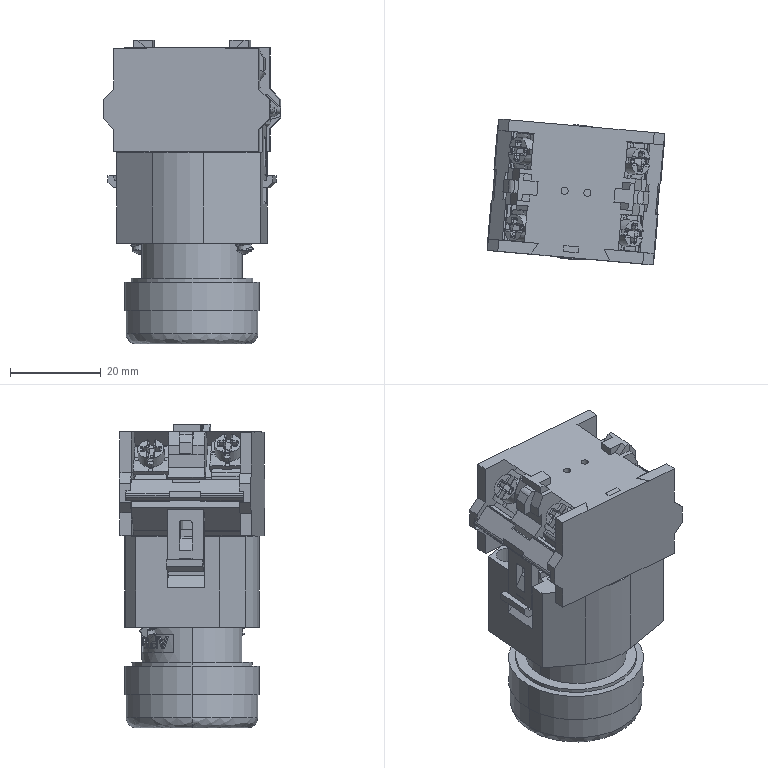Part | STEP file | 3Dcax_LA39-B2-20-y2 | 2 solids | 1700 faces | box 38.988 x 32.08 x 66.8 mm | volume 45407 mm3 | plane 1168 | spline 300 | cylinder 218 | cone 14 | commonest cylinder face diameters 3.9 x38 0.4 x25 3.2 x24 2.9 x14 0.6 x12 1.4 x12